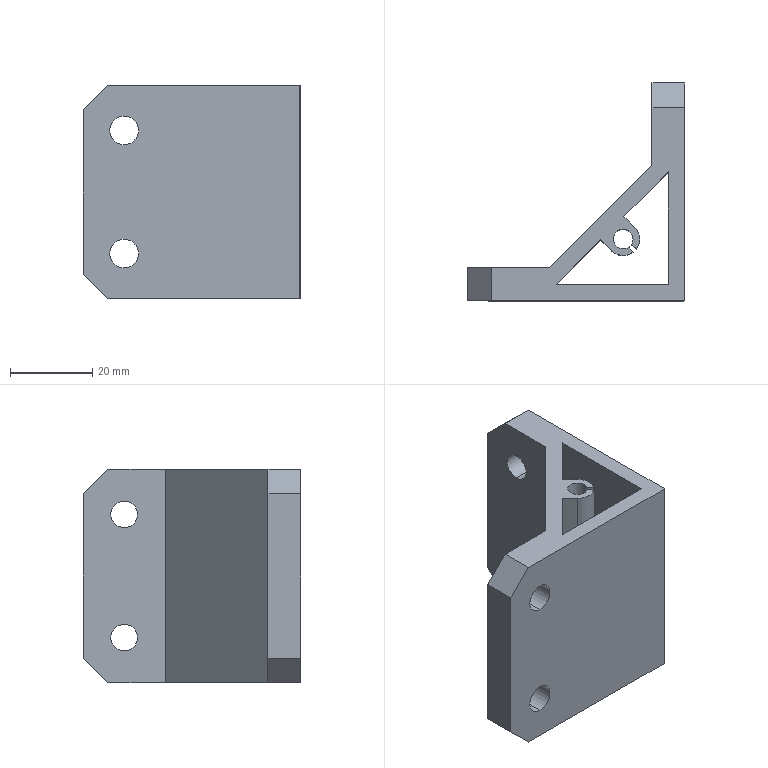Part | SolidWorks | features ICE 3, Chamfer 1, Extrusion 1 | 1 solid | 85 faces | box 53 x 53 x 52 mm | volume 37709 mm3 | plane 53 | spline 18 | cylinder 14 | commonest cylinder face diameters 6.5 x4 7 x4 4.8 x3 8 x2 0.474 x1